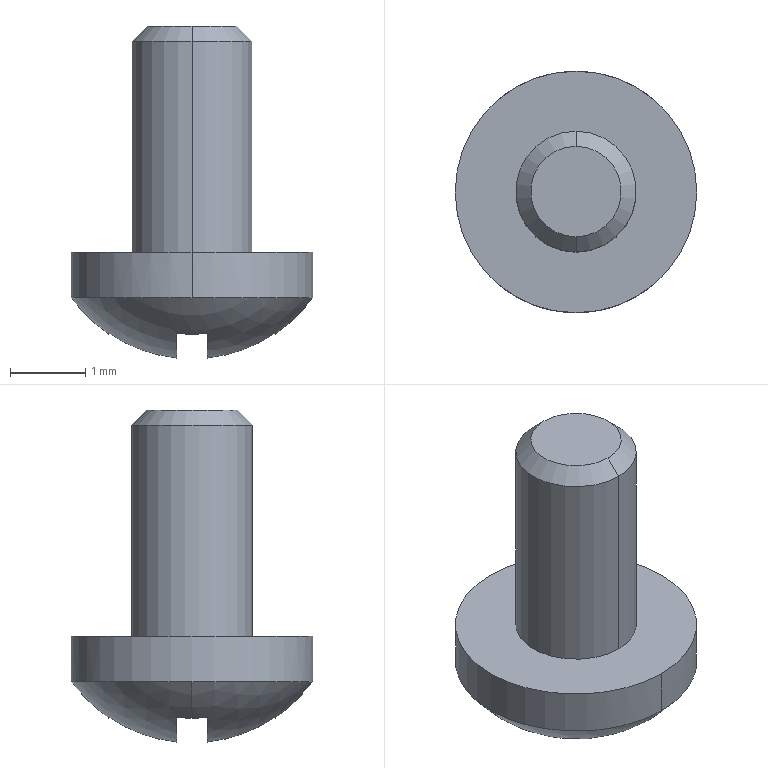Part | STEP file | ASND-0110-0160099710 | 1 solid | 23 faces | box 3.2 x 3.2 x 4.4 mm | volume 13.426 mm3 | plane 15 | cylinder 4 | cone 2 | sphere 2 | commonest cylinder face diameters 1.6 x2 3.2 x2